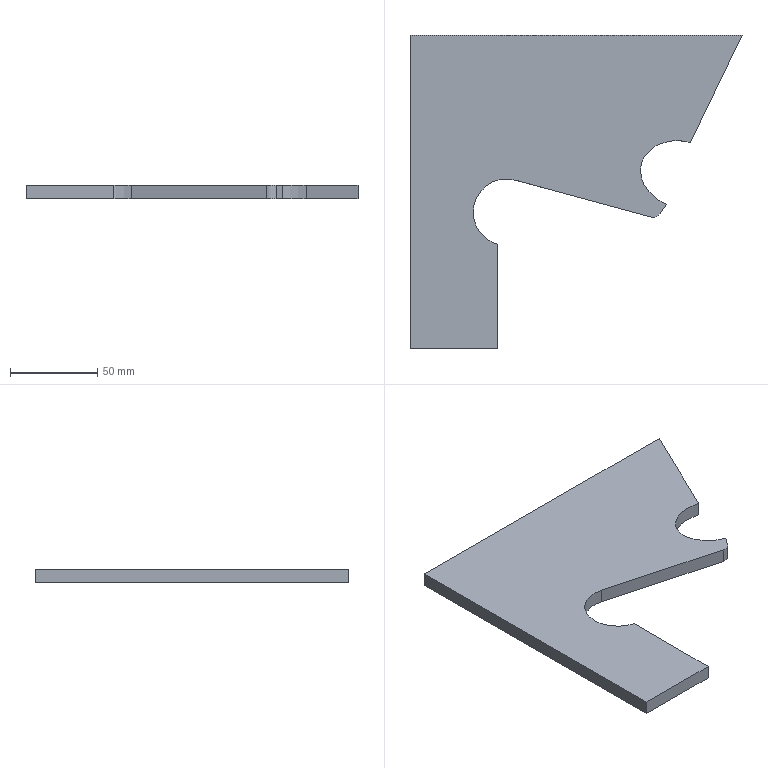Part | SolidWorks | features FlatPattern 1, SMBaseFlange 1, SheetMetal 1 | 1 solid | 14 faces | box 190.337 x 180 x 8 mm | volume 152502 mm3 | plane 9 | cylinder 3 | spline 2 | commonest cylinder face diameters 38.1 x2 10 x1
STEP:
#1=CARTESIAN_POINT('',(-117.833,32.024,8.));
#2=VERTEX_POINT('',#1);
#3=CARTESIAN_POINT('',(-89.816,44.165,8.));
#4=VERTEX_POINT('',#3);
#5=CARTESIAN_POINT('',(-117.833,32.024,8.));
#6=CARTESIAN_POINT('',(-114.912,42.794,8.));
#7=CARTESIAN_POINT('',(-103.308,47.823,8.));
#8=CARTESIAN_POINT('',(-89.816,44.165,8.));
#9=(BOUNDED_CURVE()B_SPLINE_CURVE(3,(#5,#6,#7,#8),.UNSPECIFIED.,.F.,.F.)B_SPLINE_CURVE_WITH_KNOTS((4,4),(0.,1.571),.UNSPECIFIED.)CURVE()GEOMETRIC_REPRESENTATION_ITEM()RATIONAL_B_SPLINE_CURVE((1.,0.8047,0.8047,1.))REPRESENTATION_ITEM(''));
#10=EDGE_CURVE('',#2,#4,#9,.T.);
#11=ORIENTED_EDGE('',*,*,#10,.F.);
#12=CARTESIAN_POINT('',(-117.833,32.024,0.));
#13=VERTEX_POINT('',#12);
#14=CARTESIAN_POINT('',(-117.833,32.024,8.));
#15=DIRECTION('',(0.,0.,-1.));
#16=VECTOR('',#15,1000.);
#17=LINE('',#14,#16);
#18=EDGE_CURVE('',#2,#13,#17,.T.);
#19=ORIENTED_EDGE('',*,*,#18,.T.);
#20=CARTESIAN_POINT('',(-89.816,44.165,0.));
#21=VERTEX_POINT('',#20);
#22=CARTESIAN_POINT('',(-117.833,32.024,0.));
#23=CARTESIAN_POINT('',(-114.912,42.794,0.));
#24=CARTESIAN_POINT('',(-103.308,47.823,0.));
#25=CARTESIAN_POINT('',(-89.816,44.165,0.));
#26=(BOUNDED_CURVE()B_SPLINE_CURVE(3,(#22,#23,#24,#25),.UNSPECIFIED.,.F.,.T.)B_SPLINE_CURVE_WITH_KNOTS((4,4),(0.,1.571),.UNSPECIFIED.)CURVE()GEOMETRIC_REPRESENTATION_ITEM()RATIONAL_B_SPLINE_CURVE((1.,0.8047,0.8047,1.))REPRESENTATION_ITEM(''));
#27=EDGE_CURVE('',#13,#21,#26,.T.);
#28=ORIENTED_EDGE('',*,*,#27,.T.);
#29=CARTESIAN_POINT('',(-89.816,44.165,8.));
#30=DIRECTION('',(0.,0.,-1.));
#31=VECTOR('',#30,1000.);
#32=LINE('',#29,#31);
#33=EDGE_CURVE('',#4,#21,#32,.T.);
#34=ORIENTED_EDGE('',*,*,#33,.F.);
#35=EDGE_LOOP('',(#11,#19,#28,#34));
#36=FACE_OUTER_BOUND('',#35,.T.);
#37=CARTESIAN_POINT('',(-117.833,32.024,8.));
#38=CARTESIAN_POINT('',(-117.833,32.024,0.));
#39=CARTESIAN_POINT('',(-114.912,42.794,8.));
#40=CARTESIAN_POINT('',(-114.912,42.794,0.));
#41=CARTESIAN_POINT('',(-103.308,47.823,8.));
#42=CARTESIAN_POINT('',(-103.308,47.823,0.));
#43=CARTESIAN_POINT('',(-89.816,44.165,8.));
#44=CARTESIAN_POINT('',(-89.816,44.165,0.));
#45=(BOUNDED_SURFACE()B_SPLINE_SURFACE(3,1,((#37,#38),(#39,#40),(#41,#42),(#43,#44)),.UNSPECIFIED.,.F.,.F.,.F.)B_SPLINE_SURFACE_WITH_KNOTS((4,4),(2,2),(0.,1.),(0.,1.),.UNSPECIFIED.)GEOMETRIC_REPRESENTATION_ITEM()RATIONAL_B_SPLINE_SURFACE(((1.,1.),(0.8047,0.8047),(0.8047,0.8047),(1.,1.)))REPRESENTATION_ITEM('')SURFACE());
#46=ADVANCED_FACE('',(#36),#45,.F.);
#47=CARTESIAN_POINT('',(-214.283,4.192,8.));
#48=VERTEX_POINT('',#47);
#49=CARTESIAN_POINT('',(-190.247,22.578,8.));
#50=VERTEX_POINT('',#49);
#51=CARTESIAN_POINT('',(-195.233,4.192,8.));
#52=DIRECTION('',(0.,0.,-1.));
#53=DIRECTION('',(1.,0.,0.));
#54=AXIS2_PLACEMENT_3D('',#51,#52,#53);
#55=CIRCLE('',#54,19.05);
#56=EDGE_CURVE('',#48,#50,#55,.T.);
#57=ORIENTED_EDGE('',*,*,#56,.F.);
#58=CARTESIAN_POINT('',(-214.283,4.192,0.));
#59=VERTEX_POINT('',#58);
#60=CARTESIAN_POINT('',(-214.283,4.192,8.));
#61=DIRECTION('',(0.,0.,-1.));
#62=VECTOR('',#61,1000.);
#63=LINE('',#60,#62);
#64=EDGE_CURVE('',#48,#59,#63,.T.);
#65=ORIENTED_EDGE('',*,*,#64,.T.);
#66=CARTESIAN_POINT('',(-190.247,22.578,0.));
#67=VERTEX_POINT('',#66);
#68=CARTESIAN_POINT('',(-195.233,4.192,0.));
#69=DIRECTION('',(0.,0.,-1.));
#70=DIRECTION('',(1.,0.,0.));
#71=AXIS2_PLACEMENT_3D('',#68,#69,#70);
#72=CIRCLE('',#71,19.05);
#73=EDGE_CURVE('',#59,#67,#72,.T.);
#74=ORIENTED_EDGE('',*,*,#73,.T.);
#75=CARTESIAN_POINT('',(-190.247,22.578,8.));
#76=DIRECTION('',(0.,0.,-1.));
#77=VECTOR('',#76,1000.);
#78=LINE('',#75,#77);
#79=EDGE_CURVE('',#50,#67,#78,.T.);
#80=ORIENTED_EDGE('',*,*,#79,.F.);
#81=EDGE_LOOP('',(#57,#65,#74,#80));
#82=FACE_OUTER_BOUND('',#81,.T.);
#83=CARTESIAN_POINT('',(-195.233,4.192,8.));
#84=DIRECTION('',(0.,0.,-1.));
#85=DIRECTION('',(-1.,0.,0.));
#86=AXIS2_PLACEMENT_3D('',#83,#84,#85);
#87=CYLINDRICAL_SURFACE('',#86,19.05);
#88=ADVANCED_FACE('',(#82),#87,.F.);
#89=CARTESIAN_POINT('',(-60.209,105.807,0.));
#90=VERTEX_POINT('',#89);
#91=CARTESIAN_POINT('',(-89.816,44.165,0.));
#92=DIRECTION('',(0.433,0.9014,0.));
#93=VECTOR('',#92,1000.);
#94=LINE('',#91,#93);
#95=EDGE_CURVE('',#21,#90,#94,.T.);
#96=ORIENTED_EDGE('',*,*,#95,.T.);
#97=CARTESIAN_POINT('',(-60.209,105.807,8.));
#98=VERTEX_POINT('',#97);
#99=CARTESIAN_POINT('',(-60.209,105.807,8.));
#100=DIRECTION('',(0.,0.,-1.));
#101=VECTOR('',#100,1000.);
#102=LINE('',#99,#101);
#103=EDGE_CURVE('',#98,#90,#102,.T.);
#104=ORIENTED_EDGE('',*,*,#103,.F.);
#105=CARTESIAN_POINT('',(-89.816,44.165,8.));
#106=DIRECTION('',(0.433,0.9014,0.));
#107=VECTOR('',#106,1000.);
#108=LINE('',#105,#107);
#109=EDGE_CURVE('',#4,#98,#108,.T.);
#110=ORIENTED_EDGE('',*,*,#109,.F.);
#111=ORIENTED_EDGE('',*,*,#33,.T.);
#112=EDGE_LOOP('',(#96,#104,#110,#111));
#113=FACE_OUTER_BOUND('',#112,.T.);
#114=CARTESIAN_POINT('',(-89.816,44.165,8.));
#115=DIRECTION('',(-0.9014,0.433,0.));
#116=DIRECTION('',(-0.433,-0.9014,0.));
#117=AXIS2_PLACEMENT_3D('',#114,#115,#116);
#118=PLANE('',#117);
#119=ADVANCED_FACE('',(#113),#118,.F.);
#120=CARTESIAN_POINT('',(-250.545,105.807,0.));
#121=VERTEX_POINT('',#120);
#122=CARTESIAN_POINT('',(-60.209,105.807,0.));
#123=DIRECTION('',(-1.,0.,0.));
#124=VECTOR('',#123,1000.);
#125=LINE('',#122,#124);
#126=EDGE_CURVE('',#90,#121,#125,.T.);
#127=ORIENTED_EDGE('',*,*,#126,.T.);
#128=CARTESIAN_POINT('',(-250.545,105.807,8.));
#129=VERTEX_POINT('',#128);
#130=CARTESIAN_POINT('',(-250.545,105.807,8.));
#131=DIRECTION('',(0.,0.,-1.));
#132=VECTOR('',#131,1000.);
#133=LINE('',#130,#132);
#134=EDGE_CURVE('',#129,#121,#133,.T.);
#135=ORIENTED_EDGE('',*,*,#134,.F.);
#136=CARTESIAN_POINT('',(-60.209,105.807,8.));
#137=DIRECTION('',(-1.,0.,0.));
#138=VECTOR('',#137,1000.);
#139=LINE('',#136,#138);
#140=EDGE_CURVE('',#98,#129,#139,.T.);
#141=ORIENTED_EDGE('',*,*,#140,.F.);
#142=ORIENTED_EDGE('',*,*,#103,.T.);
#143=EDGE_LOOP('',(#127,#135,#141,#142));
#144=FACE_OUTER_BOUND('',#143,.T.);
#145=CARTESIAN_POINT('',(-60.209,105.807,8.));
#146=DIRECTION('',(0.,-1.,0.));
#147=DIRECTION('',(0.,0.,-1.));
#148=AXIS2_PLACEMENT_3D('',#145,#146,#147);
#149=PLANE('',#148);
#150=ADVANCED_FACE('',(#144),#149,.F.);
#151=CARTESIAN_POINT('',(-250.545,-74.193,0.));
#152=VERTEX_POINT('',#151);
#153=CARTESIAN_POINT('',(-250.545,105.807,0.));
#154=DIRECTION('',(0.,-1.,0.));
#155=VECTOR('',#154,1000.);
#156=LINE('',#153,#155);
#157=EDGE_CURVE('',#121,#152,#156,.T.);
#158=ORIENTED_EDGE('',*,*,#157,.T.);
#159=CARTESIAN_POINT('',(-250.545,-74.193,8.));
#160=VERTEX_POINT('',#159);
#161=CARTESIAN_POINT('',(-250.545,-74.193,8.));
#162=DIRECTION('',(0.,0.,-1.));
#163=VECTOR('',#162,1000.);
#164=LINE('',#161,#163);
#165=EDGE_CURVE('',#160,#152,#164,.T.);
#166=ORIENTED_EDGE('',*,*,#165,.F.);
#167=CARTESIAN_POINT('',(-250.545,105.807,8.));
#168=DIRECTION('',(0.,-1.,0.));
#169=VECTOR('',#168,1000.);
#170=LINE('',#167,#169);
#171=EDGE_CURVE('',#129,#160,#170,.T.);
#172=ORIENTED_EDGE('',*,*,#171,.F.);
#173=ORIENTED_EDGE('',*,*,#134,.T.);
#174=EDGE_LOOP('',(#158,#166,#172,#173));
#175=FACE_OUTER_BOUND('',#174,.T.);
#176=CARTESIAN_POINT('',(-250.545,105.807,8.));
#177=DIRECTION('',(1.,0.,0.));
#178=DIRECTION('',(0.,0.,-1.));
#179=AXIS2_PLACEMENT_3D('',#176,#177,#178);
#180=PLANE('',#179);
#181=ADVANCED_FACE('',(#175),#180,.F.);
#182=CARTESIAN_POINT('',(-200.545,-74.193,0.));
#183=VERTEX_POINT('',#182);
#184=CARTESIAN_POINT('',(-200.545,-74.193,0.));
#185=DIRECTION('',(1.,0.,0.));
#186=VECTOR('',#185,1000.);
#187=LINE('',#184,#186);
#188=EDGE_CURVE('',#152,#183,#187,.T.);
#189=ORIENTED_EDGE('',*,*,#188,.T.);
#190=CARTESIAN_POINT('',(-200.545,-74.193,8.));
#191=VERTEX_POINT('',#190);
#192=CARTESIAN_POINT('',(-200.545,-74.193,8.));
#193=DIRECTION('',(0.,0.,-1.));
#194=VECTOR('',#193,1000.);
#195=LINE('',#192,#194);
#196=EDGE_CURVE('',#191,#183,#195,.T.);
#197=ORIENTED_EDGE('',*,*,#196,.F.);
#198=CARTESIAN_POINT('',(-200.545,-74.193,8.));
#199=DIRECTION('',(1.,0.,0.));
#200=VECTOR('',#199,1000.);
#201=LINE('',#198,#200);
#202=EDGE_CURVE('',#160,#191,#201,.T.);
#203=ORIENTED_EDGE('',*,*,#202,.F.);
#204=ORIENTED_EDGE('',*,*,#165,.T.);
#205=EDGE_LOOP('',(#189,#197,#203,#204));
#206=FACE_OUTER_BOUND('',#205,.T.);
#207=CARTESIAN_POINT('',(-200.545,-74.193,8.));
#208=DIRECTION('',(0.,1.,0.));
#209=DIRECTION('',(-1.,0.,0.));
#210=AXIS2_PLACEMENT_3D('',#207,#208,#209);
#211=PLANE('',#210);
#212=ADVANCED_FACE('',(#206),#211,.F.);
#213=CARTESIAN_POINT('',(-200.218,-14.194,0.));
#214=VERTEX_POINT('',#213);
#215=CARTESIAN_POINT('',(-200.545,-74.193,0.));
#216=DIRECTION('',(0.005451,1.,0.));
#217=VECTOR('',#216,1000.);
#218=LINE('',#215,#217);
#219=EDGE_CURVE('',#183,#214,#218,.T.);
#220=ORIENTED_EDGE('',*,*,#219,.T.);
#221=CARTESIAN_POINT('',(-200.218,-14.194,8.));
#222=VERTEX_POINT('',#221);
#223=CARTESIAN_POINT('',(-200.218,-14.194,8.));
#224=DIRECTION('',(0.,0.,-1.));
#225=VECTOR('',#224,1000.);
#226=LINE('',#223,#225);
#227=EDGE_CURVE('',#222,#214,#226,.T.);
#228=ORIENTED_EDGE('',*,*,#227,.F.);
#229=CARTESIAN_POINT('',(-200.545,-74.193,8.));
#230=DIRECTION('',(0.005451,1.,0.));
#231=VECTOR('',#230,1000.);
#232=LINE('',#229,#231);
#233=EDGE_CURVE('',#191,#222,#232,.T.);
#234=ORIENTED_EDGE('',*,*,#233,.F.);
#235=ORIENTED_EDGE('',*,*,#196,.T.);
#236=EDGE_LOOP('',(#220,#228,#234,#235));
#237=FACE_OUTER_BOUND('',#236,.T.);
#238=CARTESIAN_POINT('',(-200.545,-74.193,8.));
#239=DIRECTION('',(-1.,0.005451,0.));
#240=DIRECTION('',(-0.005451,-1.,0.));
#241=AXIS2_PLACEMENT_3D('',#238,#239,#240);
#242=PLANE('',#241);
#243=ADVANCED_FACE('',(#237),#242,.F.);
#244=ORIENTED_EDGE('',*,*,#64,.F.);
#245=CARTESIAN_POINT('',(-195.233,4.192,8.));
#246=DIRECTION('',(0.,0.,-1.));
#247=DIRECTION('',(1.,0.,0.));
#248=AXIS2_PLACEMENT_3D('',#245,#246,#247);
#249=CIRCLE('',#248,19.05);
#250=EDGE_CURVE('',#222,#48,#249,.T.);
#251=ORIENTED_EDGE('',*,*,#250,.F.);
#252=ORIENTED_EDGE('',*,*,#227,.T.);
#253=CARTESIAN_POINT('',(-195.233,4.192,0.));
#254=DIRECTION('',(0.,0.,-1.));
#255=DIRECTION('',(1.,0.,0.));
#256=AXIS2_PLACEMENT_3D('',#253,#254,#255);
#257=CIRCLE('',#256,19.05);
#258=EDGE_CURVE('',#214,#59,#257,.T.);
#259=ORIENTED_EDGE('',*,*,#258,.T.);
#260=EDGE_LOOP('',(#244,#251,#252,#259));
#261=FACE_OUTER_BOUND('',#260,.T.);
#262=CARTESIAN_POINT('',(-195.233,4.192,8.));
#263=DIRECTION('',(0.,0.,-1.));
#264=DIRECTION('',(-1.,0.,0.));
#265=AXIS2_PLACEMENT_3D('',#262,#263,#264);
#266=CYLINDRICAL_SURFACE('',#265,19.05);
#267=ADVANCED_FACE('',(#261),#266,.F.);
#268=CARTESIAN_POINT('',(-112.561,1.513,0.));
#269=VERTEX_POINT('',#268);
#270=CARTESIAN_POINT('',(-112.561,1.513,0.));
#271=DIRECTION('',(0.9651,-0.2617,0.));
#272=VECTOR('',#271,1000.);
#273=LINE('',#270,#272);
#274=EDGE_CURVE('',#67,#269,#273,.T.);
#275=ORIENTED_EDGE('',*,*,#274,.T.);
#276=CARTESIAN_POINT('',(-112.561,1.513,8.));
#277=VERTEX_POINT('',#276);
#278=CARTESIAN_POINT('',(-112.561,1.513,8.));
#279=DIRECTION('',(0.,0.,-1.));
#280=VECTOR('',#279,1000.);
#281=LINE('',#278,#280);
#282=EDGE_CURVE('',#277,#269,#281,.T.);
#283=ORIENTED_EDGE('',*,*,#282,.F.);
#284=CARTESIAN_POINT('',(-112.561,1.513,8.));
#285=DIRECTION('',(0.9651,-0.2617,0.));
#286=VECTOR('',#285,1000.);
#287=LINE('',#284,#286);
#288=EDGE_CURVE('',#50,#277,#287,.T.);
#289=ORIENTED_EDGE('',*,*,#288,.F.);
#290=ORIENTED_EDGE('',*,*,#79,.T.);
#291=EDGE_LOOP('',(#275,#283,#289,#290));
#292=FACE_OUTER_BOUND('',#291,.T.);
#293=CARTESIAN_POINT('',(-112.561,1.513,8.));
#294=DIRECTION('',(0.2617,0.9651,0.));
#295=DIRECTION('',(-0.9651,0.2617,0.));
#296=AXIS2_PLACEMENT_3D('',#293,#294,#295);
#297=PLANE('',#296);
#298=ADVANCED_FACE('',(#292),#297,.F.);
#299=CARTESIAN_POINT('',(-107.203,3.406,0.));
#300=VERTEX_POINT('',#299);
#301=CARTESIAN_POINT('',(-111.252,6.339,0.));
#302=DIRECTION('',(0.,0.,1.));
#303=DIRECTION('',(-1.,0.,0.));
#304=AXIS2_PLACEMENT_3D('',#301,#302,#303);
#305=CIRCLE('',#304,5.);
#306=EDGE_CURVE('',#269,#300,#305,.T.);
#307=ORIENTED_EDGE('',*,*,#306,.T.);
#308=CARTESIAN_POINT('',(-107.203,3.406,8.));
#309=VERTEX_POINT('',#308);
#310=CARTESIAN_POINT('',(-107.203,3.406,8.));
#311=DIRECTION('',(0.,0.,-1.));
#312=VECTOR('',#311,1000.);
#313=LINE('',#310,#312);
#314=EDGE_CURVE('',#309,#300,#313,.T.);
#315=ORIENTED_EDGE('',*,*,#314,.F.);
#316=CARTESIAN_POINT('',(-111.252,6.339,8.));
#317=DIRECTION('',(0.,0.,1.));
#318=DIRECTION('',(-1.,0.,0.));
#319=AXIS2_PLACEMENT_3D('',#316,#317,#318);
#320=CIRCLE('',#319,5.);
#321=EDGE_CURVE('',#277,#309,#320,.T.);
#322=ORIENTED_EDGE('',*,*,#321,.F.);
#323=ORIENTED_EDGE('',*,*,#282,.T.);
#324=EDGE_LOOP('',(#307,#315,#322,#323));
#325=FACE_OUTER_BOUND('',#324,.T.);
#326=CARTESIAN_POINT('',(-111.252,6.339,8.));
#327=DIRECTION('',(0.,0.,-1.));
#328=DIRECTION('',(-1.,0.,0.));
#329=AXIS2_PLACEMENT_3D('',#326,#327,#328);
#330=CYLINDRICAL_SURFACE('',#329,5.);
#331=ADVANCED_FACE('',(#325),#330,.T.);
#332=CARTESIAN_POINT('',(-103.417,8.633,0.));
#333=VERTEX_POINT('',#332);
#334=CARTESIAN_POINT('',(-107.203,3.406,0.));
#335=DIRECTION('',(0.5866,0.8099,0.));
#336=VECTOR('',#335,1000.);
#337=LINE('',#334,#336);
#338=EDGE_CURVE('',#300,#333,#337,.T.);
#339=ORIENTED_EDGE('',*,*,#338,.T.);
#340=CARTESIAN_POINT('',(-103.417,8.633,8.));
#341=VERTEX_POINT('',#340);
#342=CARTESIAN_POINT('',(-103.417,8.633,8.));
#343=DIRECTION('',(0.,0.,-1.));
#344=VECTOR('',#343,1000.);
#345=LINE('',#342,#344);
#346=EDGE_CURVE('',#341,#333,#345,.T.);
#347=ORIENTED_EDGE('',*,*,#346,.F.);
#348=CARTESIAN_POINT('',(-107.203,3.406,8.));
#349=DIRECTION('',(0.5866,0.8099,0.));
#350=VECTOR('',#349,1000.);
#351=LINE('',#348,#350);
#352=EDGE_CURVE('',#309,#341,#351,.T.);
#353=ORIENTED_EDGE('',*,*,#352,.F.);
#354=ORIENTED_EDGE('',*,*,#314,.T.);
#355=EDGE_LOOP('',(#339,#347,#353,#354));
#356=FACE_OUTER_BOUND('',#355,.T.);
#357=CARTESIAN_POINT('',(-107.203,3.406,8.));
#358=DIRECTION('',(-0.8099,0.5866,0.));
#359=DIRECTION('',(-0.5866,-0.8099,0.));
#360=AXIS2_PLACEMENT_3D('',#357,#358,#359);
#361=PLANE('',#360);
#362=ADVANCED_FACE('',(#356),#361,.F.);
#363=ORIENTED_EDGE('',*,*,#18,.F.);
#364=CARTESIAN_POINT('',(-103.417,8.633,8.));
#365=CARTESIAN_POINT('',(-114.68,13.312,8.));
#366=CARTESIAN_POINT('',(-120.393,22.582,8.));
#367=CARTESIAN_POINT('',(-117.833,32.024,8.));
#368=(BOUNDED_CURVE()B_SPLINE_CURVE(3,(#364,#365,#366,#367),.UNSPECIFIED.,.F.,.F.)B_SPLINE_CURVE_WITH_KNOTS((4,4),(4.874,6.283),.UNSPECIFIED.)CURVE()GEOMETRIC_REPRESENTATION_ITEM()RATIONAL_B_SPLINE_CURVE((1.,0.8411,0.8411,1.))REPRESENTATION_ITEM(''));
#369=EDGE_CURVE('',#341,#2,#368,.T.);
#370=ORIENTED_EDGE('',*,*,#369,.F.);
#371=ORIENTED_EDGE('',*,*,#346,.T.);
#372=CARTESIAN_POINT('',(-103.417,8.633,0.));
#373=CARTESIAN_POINT('',(-114.68,13.312,0.));
#374=CARTESIAN_POINT('',(-120.393,22.582,0.));
#375=CARTESIAN_POINT('',(-117.833,32.024,0.));
#376=(BOUNDED_CURVE()B_SPLINE_CURVE(3,(#372,#373,#374,#375),.UNSPECIFIED.,.F.,.F.)B_SPLINE_CURVE_WITH_KNOTS((4,4),(4.874,6.283),.UNSPECIFIED.)CURVE()GEOMETRIC_REPRESENTATION_ITEM()RATIONAL_B_SPLINE_CURVE((1.,0.8411,0.8411,1.))REPRESENTATION_ITEM(''));
#377=EDGE_CURVE('',#333,#13,#376,.T.);
#378=ORIENTED_EDGE('',*,*,#377,.T.);
#379=EDGE_LOOP('',(#363,#370,#371,#378));
#380=FACE_OUTER_BOUND('',#379,.T.);
#381=CARTESIAN_POINT('',(-103.417,8.633,8.));
#382=CARTESIAN_POINT('',(-103.417,8.633,0.));
#383=CARTESIAN_POINT('',(-114.68,13.312,8.));
#384=CARTESIAN_POINT('',(-114.68,13.312,0.));
#385=CARTESIAN_POINT('',(-120.393,22.582,8.));
#386=CARTESIAN_POINT('',(-120.393,22.582,0.));
#387=CARTESIAN_POINT('',(-117.833,32.024,8.));
#388=CARTESIAN_POINT('',(-117.833,32.024,0.));
#389=(BOUNDED_SURFACE()B_SPLINE_SURFACE(3,1,((#381,#382),(#383,#384),(#385,#386),(#387,#388)),.UNSPECIFIED.,.F.,.F.,.F.)B_SPLINE_SURFACE_WITH_KNOTS((4,4),(2,2),(0.,1.),(0.,1.),.UNSPECIFIED.)GEOMETRIC_REPRESENTATION_ITEM()RATIONAL_B_SPLINE_SURFACE(((1.,1.),(0.8411,0.8411),(0.8411,0.8411),(1.,1.)))REPRESENTATION_ITEM('')SURFACE());
#390=ADVANCED_FACE('',(#380),#389,.F.);
#391=ORIENTED_EDGE('',*,*,#109,.T.);
#392=ORIENTED_EDGE('',*,*,#140,.T.);
#393=ORIENTED_EDGE('',*,*,#171,.T.);
#394=ORIENTED_EDGE('',*,*,#202,.T.);
#395=ORIENTED_EDGE('',*,*,#233,.T.);
#396=ORIENTED_EDGE('',*,*,#250,.T.);
#397=ORIENTED_EDGE('',*,*,#56,.T.);
#398=ORIENTED_EDGE('',*,*,#288,.T.);
#399=ORIENTED_EDGE('',*,*,#321,.T.);
#400=ORIENTED_EDGE('',*,*,#352,.T.);
#401=ORIENTED_EDGE('',*,*,#369,.T.);
#402=ORIENTED_EDGE('',*,*,#10,.T.);
#403=EDGE_LOOP('',(#391,#392,#393,#394,#395,#396,#397,#398,#399,#400,#401,#402));
#404=FACE_OUTER_BOUND('',#403,.T.);
#405=CARTESIAN_POINT('',(-94.802,25.779,8.));
#406=DIRECTION('',(0.,0.,1.));
#407=DIRECTION('',(1.,0.,0.));
#408=AXIS2_PLACEMENT_3D('',#405,#406,#407);
#409=PLANE('',#408);
#410=ADVANCED_FACE('',(#404),#409,.T.);
#411=ORIENTED_EDGE('',*,*,#95,.F.);
#412=ORIENTED_EDGE('',*,*,#27,.F.);
#413=ORIENTED_EDGE('',*,*,#377,.F.);
#414=ORIENTED_EDGE('',*,*,#338,.F.);
#415=ORIENTED_EDGE('',*,*,#306,.F.);
#416=ORIENTED_EDGE('',*,*,#274,.F.);
#417=ORIENTED_EDGE('',*,*,#73,.F.);
#418=ORIENTED_EDGE('',*,*,#258,.F.);
#419=ORIENTED_EDGE('',*,*,#219,.F.);
#420=ORIENTED_EDGE('',*,*,#188,.F.);
#421=ORIENTED_EDGE('',*,*,#157,.F.);
#422=ORIENTED_EDGE('',*,*,#126,.F.);
#423=EDGE_LOOP('',(#411,#412,#413,#414,#415,#416,#417,#418,#419,#420,#421,#422));
#424=FACE_OUTER_BOUND('',#423,.T.);
#425=CARTESIAN_POINT('',(-94.802,25.779,0.));
#426=DIRECTION('',(0.,0.,1.));
#427=DIRECTION('',(1.,0.,0.));
#428=AXIS2_PLACEMENT_3D('',#425,#426,#427);
#429=PLANE('',#428);
#430=ADVANCED_FACE('',(#424),#429,.F.);
#431=CLOSED_SHELL('',(#46,#88,#119,#150,#181,#212,#243,#267,#298,#331,#362,#390,#410,#430));
#432=MANIFOLD_SOLID_BREP('',#431);
#433=CARTESIAN_POINT('',(0.,0.,0.));
#434=DIRECTION('',(0.,0.,1.));
#435=DIRECTION('',(1.,0.,0.));
#436=AXIS2_PLACEMENT_3D('',#433,#434,#435);
#437=(LENGTH_UNIT()NAMED_UNIT(*)SI_UNIT(.MILLI.,.METRE.));
#438=UNCERTAINTY_MEASURE_WITH_UNIT(LENGTH_MEASURE(0.00001),#437,'','');
#439=(NAMED_UNIT(*)PLANE_ANGLE_UNIT()SI_UNIT($,.RADIAN.));
#440=(NAMED_UNIT(*)SI_UNIT($,.STERADIAN.)SOLID_ANGLE_UNIT());
#441=(GEOMETRIC_REPRESENTATION_CONTEXT(3)GLOBAL_UNCERTAINTY_ASSIGNED_CONTEXT((#438))GLOBAL_UNIT_ASSIGNED_CONTEXT((#437,#439,#440))REPRESENTATION_CONTEXT('',''));
#442=ADVANCED_BREP_SHAPE_REPRESENTATION('',(#432,#436),#441);